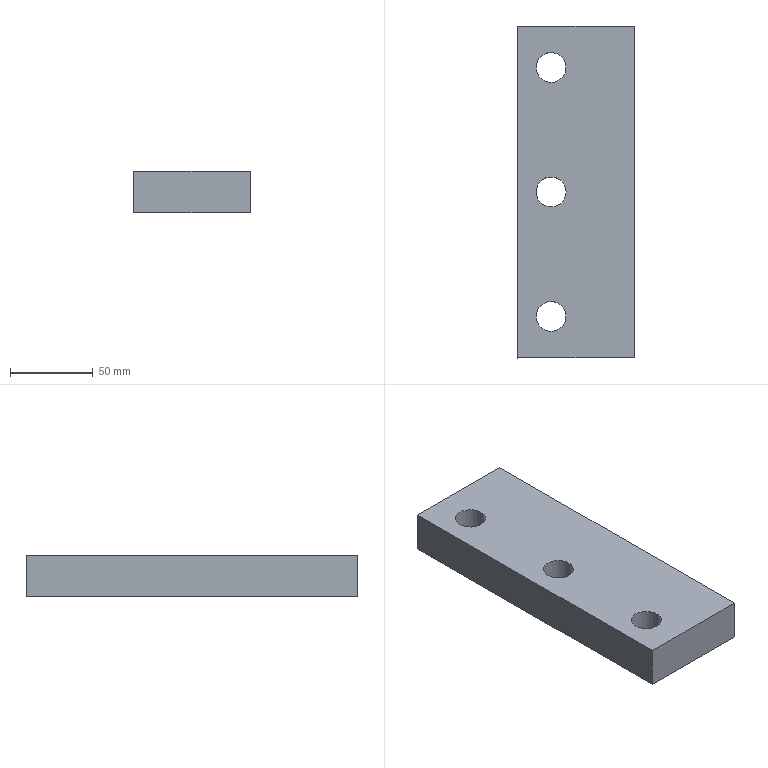Part | NX | features solid 2 | 1 solid | 9 faces | box 70 x 200 x 25 mm | volume 330915 mm3 | plane 6 | cylinder 3 | commonest cylinder face diameters 18 x3
STEP:
#1=CARTESIAN_POINT('',(-1372.,-644.605,-285.));
#2=VERTEX_POINT('',#1);
#3=CARTESIAN_POINT('',(-1372.,-644.605,-260.));
#4=VERTEX_POINT('',#3);
#5=CARTESIAN_POINT('',(-1372.,-644.605,-285.));
#6=DIRECTION('',(0.,0.,-1.));
#7=VECTOR('',#6,1000.);
#8=LINE('',#5,#7);
#9=EDGE_CURVE('',#2,#4,#8,.F.);
#10=ORIENTED_EDGE('',*,*,#9,.F.);
#11=CARTESIAN_POINT('',(-1372.,-844.605,-285.));
#12=VERTEX_POINT('',#11);
#13=CARTESIAN_POINT('',(-1372.,-814.605,-285.));
#14=DIRECTION('',(0.,1.,0.));
#15=VECTOR('',#14,1000.);
#16=LINE('',#13,#15);
#17=EDGE_CURVE('',#12,#2,#16,.T.);
#18=ORIENTED_EDGE('',*,*,#17,.F.);
#19=CARTESIAN_POINT('',(-1372.,-844.605,-260.));
#20=VERTEX_POINT('',#19);
#21=CARTESIAN_POINT('',(-1372.,-844.605,-285.));
#22=DIRECTION('',(0.,0.,-1.));
#23=VECTOR('',#22,1000.);
#24=LINE('',#21,#23);
#25=EDGE_CURVE('',#12,#20,#24,.F.);
#26=ORIENTED_EDGE('',*,*,#25,.T.);
#27=CARTESIAN_POINT('',(-1372.,-814.605,-260.));
#28=DIRECTION('',(0.,1.,0.));
#29=VECTOR('',#28,1000.);
#30=LINE('',#27,#29);
#31=EDGE_CURVE('',#20,#4,#30,.T.);
#32=ORIENTED_EDGE('',*,*,#31,.T.);
#33=EDGE_LOOP('',(#10,#18,#26,#32));
#34=FACE_BOUND('',#33,.T.);
#35=CARTESIAN_POINT('',(-1372.,-814.605,-285.));
#36=DIRECTION('',(-1.,0.,0.));
#37=DIRECTION('',(0.,1.,0.));
#38=AXIS2_PLACEMENT_3D('',#35,#36,#37);
#39=PLANE('',#38);
#40=ADVANCED_FACE('',(#34),#39,.T.);
#41=ORIENTED_EDGE('',*,*,#25,.F.);
#42=CARTESIAN_POINT('',(-1302.,-844.605,-285.));
#43=VERTEX_POINT('',#42);
#44=CARTESIAN_POINT('',(-1372.,-844.605,-285.));
#45=DIRECTION('',(1.,0.,0.));
#46=VECTOR('',#45,1000.);
#47=LINE('',#44,#46);
#48=EDGE_CURVE('',#12,#43,#47,.T.);
#49=ORIENTED_EDGE('',*,*,#48,.T.);
#50=CARTESIAN_POINT('',(-1302.,-844.605,-260.));
#51=VERTEX_POINT('',#50);
#52=CARTESIAN_POINT('',(-1302.,-844.605,-285.));
#53=DIRECTION('',(0.,0.,-1.));
#54=VECTOR('',#53,1000.);
#55=LINE('',#52,#54);
#56=EDGE_CURVE('',#43,#51,#55,.F.);
#57=ORIENTED_EDGE('',*,*,#56,.T.);
#58=CARTESIAN_POINT('',(-1372.,-844.605,-260.));
#59=DIRECTION('',(1.,0.,0.));
#60=VECTOR('',#59,1000.);
#61=LINE('',#58,#60);
#62=EDGE_CURVE('',#20,#51,#61,.T.);
#63=ORIENTED_EDGE('',*,*,#62,.F.);
#64=EDGE_LOOP('',(#41,#49,#57,#63));
#65=FACE_BOUND('',#64,.T.);
#66=CARTESIAN_POINT('',(-1372.,-844.605,-285.));
#67=DIRECTION('',(0.,1.,0.));
#68=DIRECTION('',(1.,0.,0.));
#69=AXIS2_PLACEMENT_3D('',#66,#67,#68);
#70=PLANE('',#69);
#71=ADVANCED_FACE('',(#65),#70,.F.);
#72=ORIENTED_EDGE('',*,*,#56,.F.);
#73=CARTESIAN_POINT('',(-1302.,-644.605,-285.));
#74=VERTEX_POINT('',#73);
#75=CARTESIAN_POINT('',(-1302.,-814.605,-285.));
#76=DIRECTION('',(0.,1.,0.));
#77=VECTOR('',#76,1000.);
#78=LINE('',#75,#77);
#79=EDGE_CURVE('',#43,#74,#78,.T.);
#80=ORIENTED_EDGE('',*,*,#79,.T.);
#81=CARTESIAN_POINT('',(-1302.,-644.605,-260.));
#82=VERTEX_POINT('',#81);
#83=CARTESIAN_POINT('',(-1302.,-644.605,-285.));
#84=DIRECTION('',(0.,0.,-1.));
#85=VECTOR('',#84,1000.);
#86=LINE('',#83,#85);
#87=EDGE_CURVE('',#74,#82,#86,.F.);
#88=ORIENTED_EDGE('',*,*,#87,.T.);
#89=CARTESIAN_POINT('',(-1302.,-814.605,-260.));
#90=DIRECTION('',(0.,1.,0.));
#91=VECTOR('',#90,1000.);
#92=LINE('',#89,#91);
#93=EDGE_CURVE('',#51,#82,#92,.T.);
#94=ORIENTED_EDGE('',*,*,#93,.F.);
#95=EDGE_LOOP('',(#72,#80,#88,#94));
#96=FACE_BOUND('',#95,.T.);
#97=CARTESIAN_POINT('',(-1302.,-814.605,-285.));
#98=DIRECTION('',(-1.,0.,0.));
#99=DIRECTION('',(0.,1.,0.));
#100=AXIS2_PLACEMENT_3D('',#97,#98,#99);
#101=PLANE('',#100);
#102=ADVANCED_FACE('',(#96),#101,.F.);
#103=CARTESIAN_POINT('',(-1372.,-644.605,-285.));
#104=DIRECTION('',(1.,0.,0.));
#105=VECTOR('',#104,1000.);
#106=LINE('',#103,#105);
#107=EDGE_CURVE('',#2,#74,#106,.T.);
#108=ORIENTED_EDGE('',*,*,#107,.F.);
#109=ORIENTED_EDGE('',*,*,#9,.T.);
#110=CARTESIAN_POINT('',(-1372.,-644.605,-260.));
#111=DIRECTION('',(1.,0.,0.));
#112=VECTOR('',#111,1000.);
#113=LINE('',#110,#112);
#114=EDGE_CURVE('',#4,#82,#113,.T.);
#115=ORIENTED_EDGE('',*,*,#114,.T.);
#116=ORIENTED_EDGE('',*,*,#87,.F.);
#117=EDGE_LOOP('',(#108,#109,#115,#116));
#118=FACE_BOUND('',#117,.T.);
#119=CARTESIAN_POINT('',(-1372.,-644.605,-285.));
#120=DIRECTION('',(0.,1.,0.));
#121=DIRECTION('',(1.,0.,0.));
#122=AXIS2_PLACEMENT_3D('',#119,#120,#121);
#123=PLANE('',#122);
#124=ADVANCED_FACE('',(#118),#123,.T.);
#125=CARTESIAN_POINT('',(-1343.,-744.605,-260.));
#126=VERTEX_POINT('',#125);
#127=CARTESIAN_POINT('',(-1352.,-744.605,-260.));
#128=DIRECTION('',(0.,0.,1.));
#129=DIRECTION('',(1.,0.,0.));
#130=AXIS2_PLACEMENT_3D('',#127,#128,#129);
#131=CIRCLE('',#130,9.);
#132=EDGE_CURVE('',#126,#126,#131,.T.);
#133=ORIENTED_EDGE('',*,*,#132,.F.);
#134=EDGE_LOOP('',(#133));
#135=FACE_BOUND('',#134,.T.);
#136=CARTESIAN_POINT('',(-1354.255,-678.318,-260.));
#137=VERTEX_POINT('',#136);
#138=CARTESIAN_POINT('',(-1352.,-669.605,-260.));
#139=DIRECTION('',(0.,0.,1.));
#140=DIRECTION('',(-0.2506,-0.9681,0.));
#141=AXIS2_PLACEMENT_3D('',#138,#139,#140);
#142=CIRCLE('',#141,9.);
#143=EDGE_CURVE('',#137,#137,#142,.T.);
#144=ORIENTED_EDGE('',*,*,#143,.F.);
#145=EDGE_LOOP('',(#144));
#146=FACE_BOUND('',#145,.T.);
#147=CARTESIAN_POINT('',(-1354.255,-828.318,-260.));
#148=VERTEX_POINT('',#147);
#149=CARTESIAN_POINT('',(-1352.,-819.605,-260.));
#150=DIRECTION('',(0.,0.,1.));
#151=DIRECTION('',(-0.2506,-0.9681,0.));
#152=AXIS2_PLACEMENT_3D('',#149,#150,#151);
#153=CIRCLE('',#152,9.);
#154=EDGE_CURVE('',#148,#148,#153,.T.);
#155=ORIENTED_EDGE('',*,*,#154,.F.);
#156=EDGE_LOOP('',(#155));
#157=FACE_BOUND('',#156,.T.);
#158=ORIENTED_EDGE('',*,*,#93,.T.);
#159=ORIENTED_EDGE('',*,*,#114,.F.);
#160=ORIENTED_EDGE('',*,*,#31,.F.);
#161=ORIENTED_EDGE('',*,*,#62,.T.);
#162=EDGE_LOOP('',(#158,#159,#160,#161));
#163=FACE_BOUND('',#162,.T.);
#164=CARTESIAN_POINT('',(-1372.,-814.605,-260.));
#165=DIRECTION('',(0.,0.,1.));
#166=DIRECTION('',(0.2506,0.9681,0.));
#167=AXIS2_PLACEMENT_3D('',#164,#165,#166);
#168=PLANE('',#167);
#169=ADVANCED_FACE('',(#135,#146,#157,#163),#168,.T.);
#170=CARTESIAN_POINT('',(-1343.,-744.605,-285.));
#171=VERTEX_POINT('',#170);
#172=CARTESIAN_POINT('',(-1352.,-744.605,-285.));
#173=DIRECTION('',(0.,0.,1.));
#174=DIRECTION('',(1.,0.,0.));
#175=AXIS2_PLACEMENT_3D('',#172,#173,#174);
#176=CIRCLE('',#175,9.);
#177=EDGE_CURVE('',#171,#171,#176,.T.);
#178=ORIENTED_EDGE('',*,*,#177,.T.);
#179=EDGE_LOOP('',(#178));
#180=FACE_BOUND('',#179,.T.);
#181=CARTESIAN_POINT('',(-1349.745,-660.892,-285.));
#182=VERTEX_POINT('',#181);
#183=CARTESIAN_POINT('',(-1352.,-669.605,-285.));
#184=DIRECTION('',(0.,0.,-1.));
#185=DIRECTION('',(0.2506,0.9681,0.));
#186=AXIS2_PLACEMENT_3D('',#183,#184,#185);
#187=CIRCLE('',#186,9.);
#188=EDGE_CURVE('',#182,#182,#187,.T.);
#189=ORIENTED_EDGE('',*,*,#188,.F.);
#190=EDGE_LOOP('',(#189));
#191=FACE_BOUND('',#190,.T.);
#192=CARTESIAN_POINT('',(-1349.745,-810.892,-285.));
#193=VERTEX_POINT('',#192);
#194=CARTESIAN_POINT('',(-1352.,-819.605,-285.));
#195=DIRECTION('',(0.,0.,-1.));
#196=DIRECTION('',(0.2506,0.9681,0.));
#197=AXIS2_PLACEMENT_3D('',#194,#195,#196);
#198=CIRCLE('',#197,9.);
#199=EDGE_CURVE('',#193,#193,#198,.T.);
#200=ORIENTED_EDGE('',*,*,#199,.F.);
#201=EDGE_LOOP('',(#200));
#202=FACE_BOUND('',#201,.T.);
#203=ORIENTED_EDGE('',*,*,#79,.F.);
#204=ORIENTED_EDGE('',*,*,#48,.F.);
#205=ORIENTED_EDGE('',*,*,#17,.T.);
#206=ORIENTED_EDGE('',*,*,#107,.T.);
#207=EDGE_LOOP('',(#203,#204,#205,#206));
#208=FACE_BOUND('',#207,.T.);
#209=CARTESIAN_POINT('',(-1372.,-814.605,-285.));
#210=DIRECTION('',(0.,0.,1.));
#211=DIRECTION('',(0.2506,0.9681,0.));
#212=AXIS2_PLACEMENT_3D('',#209,#210,#211);
#213=PLANE('',#212);
#214=ADVANCED_FACE('',(#180,#191,#202,#208),#213,.F.);
#215=ORIENTED_EDGE('',*,*,#154,.T.);
#216=EDGE_LOOP('',(#215));
#217=FACE_BOUND('',#216,.T.);
#218=ORIENTED_EDGE('',*,*,#199,.T.);
#219=EDGE_LOOP('',(#218));
#220=FACE_BOUND('',#219,.T.);
#221=CARTESIAN_POINT('',(-1352.,-819.605,-260.));
#222=DIRECTION('',(0.,0.,-1.));
#223=DIRECTION('',(-0.2506,-0.9681,0.));
#224=AXIS2_PLACEMENT_3D('',#221,#222,#223);
#225=CYLINDRICAL_SURFACE('',#224,9.);
#226=ADVANCED_FACE('',(#217,#220),#225,.F.);
#227=ORIENTED_EDGE('',*,*,#143,.T.);
#228=EDGE_LOOP('',(#227));
#229=FACE_BOUND('',#228,.T.);
#230=ORIENTED_EDGE('',*,*,#188,.T.);
#231=EDGE_LOOP('',(#230));
#232=FACE_BOUND('',#231,.T.);
#233=CARTESIAN_POINT('',(-1352.,-669.605,-260.));
#234=DIRECTION('',(0.,0.,-1.));
#235=DIRECTION('',(-0.2506,-0.9681,0.));
#236=AXIS2_PLACEMENT_3D('',#233,#234,#235);
#237=CYLINDRICAL_SURFACE('',#236,9.);
#238=ADVANCED_FACE('',(#229,#232),#237,.F.);
#239=ORIENTED_EDGE('',*,*,#132,.T.);
#240=EDGE_LOOP('',(#239));
#241=FACE_BOUND('',#240,.T.);
#242=ORIENTED_EDGE('',*,*,#177,.F.);
#243=EDGE_LOOP('',(#242));
#244=FACE_BOUND('',#243,.T.);
#245=CARTESIAN_POINT('',(-1352.,-744.605,-460.));
#246=DIRECTION('',(0.,0.,1.));
#247=DIRECTION('',(1.,0.,0.));
#248=AXIS2_PLACEMENT_3D('',#245,#246,#247);
#249=CYLINDRICAL_SURFACE('',#248,9.);
#250=ADVANCED_FACE('',(#241,#244),#249,.F.);
#251=CLOSED_SHELL('',(#40,#71,#102,#124,#169,#214,#226,#238,#250));
#252=MANIFOLD_SOLID_BREP('',#251);
#253=(LENGTH_UNIT()NAMED_UNIT(*)SI_UNIT(.MILLI.,.METRE.));
#254=UNCERTAINTY_MEASURE_WITH_UNIT(LENGTH_MEASURE(0.00001),#253,'','');
#255=(NAMED_UNIT(*)PLANE_ANGLE_UNIT()SI_UNIT($,.RADIAN.));
#256=(NAMED_UNIT(*)SI_UNIT($,.STERADIAN.)SOLID_ANGLE_UNIT());
#257=(GEOMETRIC_REPRESENTATION_CONTEXT(3)GLOBAL_UNCERTAINTY_ASSIGNED_CONTEXT((#254))GLOBAL_UNIT_ASSIGNED_CONTEXT((#253,#255,#256))REPRESENTATION_CONTEXT('',''));
#258=ADVANCED_BREP_SHAPE_REPRESENTATION('',(#252),#257);